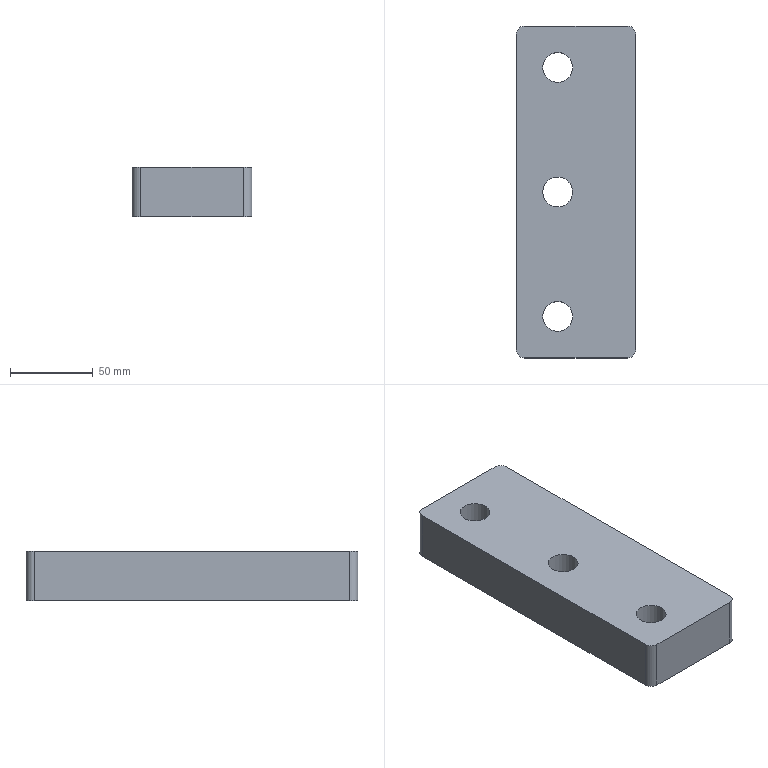Part | NX | features MAIN_BODY 2 | 1 solid | 13 faces | box 72 x 200 x 30 mm | volume 408454 mm3 | cylinder 7 | plane 6 | commonest cylinder face diameters 10 x4 18 x3
STEP:
#1=CARTESIAN_POINT('',(-700.,785.001,85.));
#2=VERTEX_POINT('',#1);
#3=CARTESIAN_POINT('',(-762.,785.001,85.));
#4=VERTEX_POINT('',#3);
#5=CARTESIAN_POINT('',(-695.,785.001,85.));
#6=DIRECTION('',(-1.,0.,0.));
#7=VECTOR('',#6,1000.);
#8=LINE('',#5,#7);
#9=EDGE_CURVE('',#2,#4,#8,.T.);
#10=ORIENTED_EDGE('',*,*,#9,.F.);
#11=CARTESIAN_POINT('',(-700.,785.001,55.));
#12=VERTEX_POINT('',#11);
#13=CARTESIAN_POINT('',(-700.,785.001,55.));
#14=DIRECTION('',(0.,0.,1.));
#15=VECTOR('',#14,1000.);
#16=LINE('',#13,#15);
#17=EDGE_CURVE('',#2,#12,#16,.F.);
#18=ORIENTED_EDGE('',*,*,#17,.T.);
#19=CARTESIAN_POINT('',(-762.,785.001,55.));
#20=VERTEX_POINT('',#19);
#21=CARTESIAN_POINT('',(-695.,785.001,55.));
#22=DIRECTION('',(-1.,0.,0.));
#23=VECTOR('',#22,1000.);
#24=LINE('',#21,#23);
#25=EDGE_CURVE('',#12,#20,#24,.T.);
#26=ORIENTED_EDGE('',*,*,#25,.T.);
#27=CARTESIAN_POINT('',(-762.,785.001,55.));
#28=DIRECTION('',(0.,0.,1.));
#29=VECTOR('',#28,1000.);
#30=LINE('',#27,#29);
#31=EDGE_CURVE('',#20,#4,#30,.T.);
#32=ORIENTED_EDGE('',*,*,#31,.T.);
#33=EDGE_LOOP('',(#10,#18,#26,#32));
#34=FACE_BOUND('',#33,.T.);
#35=CARTESIAN_POINT('',(-695.,785.001,55.));
#36=DIRECTION('',(0.,1.,0.));
#37=DIRECTION('',(1.,0.,0.));
#38=AXIS2_PLACEMENT_3D('',#35,#36,#37);
#39=PLANE('',#38);
#40=ADVANCED_FACE('',(#34),#39,.T.);
#41=CARTESIAN_POINT('',(-767.,780.001,85.));
#42=VERTEX_POINT('',#41);
#43=CARTESIAN_POINT('',(-767.,590.001,85.));
#44=VERTEX_POINT('',#43);
#45=CARTESIAN_POINT('',(-767.,785.001,85.));
#46=DIRECTION('',(0.,-1.,0.));
#47=VECTOR('',#46,1000.);
#48=LINE('',#45,#47);
#49=EDGE_CURVE('',#42,#44,#48,.T.);
#50=ORIENTED_EDGE('',*,*,#49,.F.);
#51=CARTESIAN_POINT('',(-767.,780.001,55.));
#52=VERTEX_POINT('',#51);
#53=CARTESIAN_POINT('',(-767.,780.001,55.));
#54=DIRECTION('',(0.,0.,1.));
#55=VECTOR('',#54,1000.);
#56=LINE('',#53,#55);
#57=EDGE_CURVE('',#42,#52,#56,.F.);
#58=ORIENTED_EDGE('',*,*,#57,.T.);
#59=CARTESIAN_POINT('',(-767.,590.001,55.));
#60=VERTEX_POINT('',#59);
#61=CARTESIAN_POINT('',(-767.,785.001,55.));
#62=DIRECTION('',(0.,-1.,0.));
#63=VECTOR('',#62,1000.);
#64=LINE('',#61,#63);
#65=EDGE_CURVE('',#52,#60,#64,.T.);
#66=ORIENTED_EDGE('',*,*,#65,.T.);
#67=CARTESIAN_POINT('',(-767.,590.001,55.));
#68=DIRECTION('',(0.,0.,1.));
#69=VECTOR('',#68,1000.);
#70=LINE('',#67,#69);
#71=EDGE_CURVE('',#60,#44,#70,.T.);
#72=ORIENTED_EDGE('',*,*,#71,.T.);
#73=EDGE_LOOP('',(#50,#58,#66,#72));
#74=FACE_BOUND('',#73,.T.);
#75=CARTESIAN_POINT('',(-767.,785.001,55.));
#76=DIRECTION('',(-1.,0.,0.));
#77=DIRECTION('',(0.,1.,0.));
#78=AXIS2_PLACEMENT_3D('',#75,#76,#77);
#79=PLANE('',#78);
#80=ADVANCED_FACE('',(#74),#79,.T.);
#81=CARTESIAN_POINT('',(-695.,590.001,55.));
#82=VERTEX_POINT('',#81);
#83=CARTESIAN_POINT('',(-695.,780.001,55.));
#84=VERTEX_POINT('',#83);
#85=CARTESIAN_POINT('',(-695.,685.001,55.));
#86=DIRECTION('',(0.,1.,0.));
#87=VECTOR('',#86,1000.);
#88=LINE('',#85,#87);
#89=EDGE_CURVE('',#82,#84,#88,.T.);
#90=ORIENTED_EDGE('',*,*,#89,.T.);
#91=CARTESIAN_POINT('',(-695.,780.001,85.));
#92=VERTEX_POINT('',#91);
#93=CARTESIAN_POINT('',(-695.,780.001,55.));
#94=DIRECTION('',(0.,0.,1.));
#95=VECTOR('',#94,1000.);
#96=LINE('',#93,#95);
#97=EDGE_CURVE('',#84,#92,#96,.T.);
#98=ORIENTED_EDGE('',*,*,#97,.T.);
#99=CARTESIAN_POINT('',(-695.,590.001,85.));
#100=VERTEX_POINT('',#99);
#101=CARTESIAN_POINT('',(-695.,685.001,85.));
#102=DIRECTION('',(0.,1.,0.));
#103=VECTOR('',#102,1000.);
#104=LINE('',#101,#103);
#105=EDGE_CURVE('',#100,#92,#104,.T.);
#106=ORIENTED_EDGE('',*,*,#105,.F.);
#107=CARTESIAN_POINT('',(-695.,590.001,55.));
#108=DIRECTION('',(0.,0.,1.));
#109=VECTOR('',#108,1000.);
#110=LINE('',#107,#109);
#111=EDGE_CURVE('',#100,#82,#110,.F.);
#112=ORIENTED_EDGE('',*,*,#111,.T.);
#113=EDGE_LOOP('',(#90,#98,#106,#112));
#114=FACE_BOUND('',#113,.T.);
#115=CARTESIAN_POINT('',(-695.,685.001,55.));
#116=DIRECTION('',(1.,0.,0.));
#117=DIRECTION('',(0.,0.,-1.));
#118=AXIS2_PLACEMENT_3D('',#115,#116,#117);
#119=PLANE('',#118);
#120=ADVANCED_FACE('',(#114),#119,.T.);
#121=ORIENTED_EDGE('',*,*,#25,.F.);
#122=CARTESIAN_POINT('',(-700.,780.001,55.));
#123=DIRECTION('',(0.,0.,1.));
#124=DIRECTION('',(0.,-1.,0.));
#125=AXIS2_PLACEMENT_3D('',#122,#123,#124);
#126=CIRCLE('',#125,5.);
#127=EDGE_CURVE('',#12,#84,#126,.F.);
#128=ORIENTED_EDGE('',*,*,#127,.T.);
#129=ORIENTED_EDGE('',*,*,#89,.F.);
#130=CARTESIAN_POINT('',(-700.,585.001,55.));
#131=VERTEX_POINT('',#130);
#132=CARTESIAN_POINT('',(-700.,590.001,55.));
#133=DIRECTION('',(0.,0.,1.));
#134=DIRECTION('',(0.,-1.,0.));
#135=AXIS2_PLACEMENT_3D('',#132,#133,#134);
#136=CIRCLE('',#135,5.);
#137=EDGE_CURVE('',#82,#131,#136,.F.);
#138=ORIENTED_EDGE('',*,*,#137,.T.);
#139=CARTESIAN_POINT('',(-762.,585.001,55.));
#140=VERTEX_POINT('',#139);
#141=CARTESIAN_POINT('',(-695.,585.001,55.));
#142=DIRECTION('',(-1.,0.,0.));
#143=VECTOR('',#142,1000.);
#144=LINE('',#141,#143);
#145=EDGE_CURVE('',#131,#140,#144,.T.);
#146=ORIENTED_EDGE('',*,*,#145,.T.);
#147=CARTESIAN_POINT('',(-762.,590.001,55.));
#148=DIRECTION('',(0.,0.,1.));
#149=DIRECTION('',(0.,-1.,0.));
#150=AXIS2_PLACEMENT_3D('',#147,#148,#149);
#151=CIRCLE('',#150,5.);
#152=EDGE_CURVE('',#140,#60,#151,.F.);
#153=ORIENTED_EDGE('',*,*,#152,.T.);
#154=ORIENTED_EDGE('',*,*,#65,.F.);
#155=CARTESIAN_POINT('',(-762.,780.001,55.));
#156=DIRECTION('',(0.,0.,1.));
#157=DIRECTION('',(0.,-1.,0.));
#158=AXIS2_PLACEMENT_3D('',#155,#156,#157);
#159=CIRCLE('',#158,5.);
#160=EDGE_CURVE('',#52,#20,#159,.F.);
#161=ORIENTED_EDGE('',*,*,#160,.T.);
#162=EDGE_LOOP('',(#121,#128,#129,#138,#146,#153,#154,#161));
#163=FACE_BOUND('',#162,.T.);
#164=CARTESIAN_POINT('',(-742.,751.001,55.));
#165=VERTEX_POINT('',#164);
#166=CARTESIAN_POINT('',(-742.,760.001,55.));
#167=DIRECTION('',(0.,0.,1.));
#168=DIRECTION('',(0.,-1.,0.));
#169=AXIS2_PLACEMENT_3D('',#166,#167,#168);
#170=CIRCLE('',#169,9.);
#171=EDGE_CURVE('',#165,#165,#170,.T.);
#172=ORIENTED_EDGE('',*,*,#171,.T.);
#173=EDGE_LOOP('',(#172));
#174=FACE_BOUND('',#173,.T.);
#175=CARTESIAN_POINT('',(-742.,676.001,55.));
#176=VERTEX_POINT('',#175);
#177=CARTESIAN_POINT('',(-742.,685.001,55.));
#178=DIRECTION('',(0.,0.,1.));
#179=DIRECTION('',(0.,-1.,0.));
#180=AXIS2_PLACEMENT_3D('',#177,#178,#179);
#181=CIRCLE('',#180,9.);
#182=EDGE_CURVE('',#176,#176,#181,.T.);
#183=ORIENTED_EDGE('',*,*,#182,.T.);
#184=EDGE_LOOP('',(#183));
#185=FACE_BOUND('',#184,.T.);
#186=CARTESIAN_POINT('',(-742.,619.001,55.));
#187=VERTEX_POINT('',#186);
#188=CARTESIAN_POINT('',(-742.,610.001,55.));
#189=DIRECTION('',(0.,0.,-1.));
#190=DIRECTION('',(0.,1.,0.));
#191=AXIS2_PLACEMENT_3D('',#188,#189,#190);
#192=CIRCLE('',#191,9.);
#193=EDGE_CURVE('',#187,#187,#192,.T.);
#194=ORIENTED_EDGE('',*,*,#193,.F.);
#195=EDGE_LOOP('',(#194));
#196=FACE_BOUND('',#195,.T.);
#197=CARTESIAN_POINT('',(-767.,785.001,55.));
#198=DIRECTION('',(0.,0.,1.));
#199=DIRECTION('',(0.,-1.,0.));
#200=AXIS2_PLACEMENT_3D('',#197,#198,#199);
#201=PLANE('',#200);
#202=ADVANCED_FACE('',(#163,#174,#185,#196),#201,.F.);
#203=ORIENTED_EDGE('',*,*,#105,.T.);
#204=CARTESIAN_POINT('',(-700.,780.001,85.));
#205=DIRECTION('',(0.,0.,1.));
#206=DIRECTION('',(0.,-1.,0.));
#207=AXIS2_PLACEMENT_3D('',#204,#205,#206);
#208=CIRCLE('',#207,5.);
#209=EDGE_CURVE('',#92,#2,#208,.T.);
#210=ORIENTED_EDGE('',*,*,#209,.T.);
#211=ORIENTED_EDGE('',*,*,#9,.T.);
#212=CARTESIAN_POINT('',(-762.,780.001,85.));
#213=DIRECTION('',(0.,0.,1.));
#214=DIRECTION('',(0.,-1.,0.));
#215=AXIS2_PLACEMENT_3D('',#212,#213,#214);
#216=CIRCLE('',#215,5.);
#217=EDGE_CURVE('',#4,#42,#216,.T.);
#218=ORIENTED_EDGE('',*,*,#217,.T.);
#219=ORIENTED_EDGE('',*,*,#49,.T.);
#220=CARTESIAN_POINT('',(-762.,585.001,85.));
#221=VERTEX_POINT('',#220);
#222=CARTESIAN_POINT('',(-762.,590.001,85.));
#223=DIRECTION('',(0.,0.,1.));
#224=DIRECTION('',(0.,-1.,0.));
#225=AXIS2_PLACEMENT_3D('',#222,#223,#224);
#226=CIRCLE('',#225,5.);
#227=EDGE_CURVE('',#44,#221,#226,.T.);
#228=ORIENTED_EDGE('',*,*,#227,.T.);
#229=CARTESIAN_POINT('',(-700.,585.001,85.));
#230=VERTEX_POINT('',#229);
#231=CARTESIAN_POINT('',(-695.,585.001,85.));
#232=DIRECTION('',(-1.,0.,0.));
#233=VECTOR('',#232,1000.);
#234=LINE('',#231,#233);
#235=EDGE_CURVE('',#230,#221,#234,.T.);
#236=ORIENTED_EDGE('',*,*,#235,.F.);
#237=CARTESIAN_POINT('',(-700.,590.001,85.));
#238=DIRECTION('',(0.,0.,1.));
#239=DIRECTION('',(0.,-1.,0.));
#240=AXIS2_PLACEMENT_3D('',#237,#238,#239);
#241=CIRCLE('',#240,5.);
#242=EDGE_CURVE('',#230,#100,#241,.T.);
#243=ORIENTED_EDGE('',*,*,#242,.T.);
#244=EDGE_LOOP('',(#203,#210,#211,#218,#219,#228,#236,#243));
#245=FACE_BOUND('',#244,.T.);
#246=CARTESIAN_POINT('',(-742.,676.001,85.));
#247=VERTEX_POINT('',#246);
#248=CARTESIAN_POINT('',(-742.,685.001,85.));
#249=DIRECTION('',(0.,0.,1.));
#250=DIRECTION('',(0.,-1.,0.));
#251=AXIS2_PLACEMENT_3D('',#248,#249,#250);
#252=CIRCLE('',#251,9.);
#253=EDGE_CURVE('',#247,#247,#252,.T.);
#254=ORIENTED_EDGE('',*,*,#253,.F.);
#255=EDGE_LOOP('',(#254));
#256=FACE_BOUND('',#255,.T.);
#257=CARTESIAN_POINT('',(-742.,751.001,85.));
#258=VERTEX_POINT('',#257);
#259=CARTESIAN_POINT('',(-742.,760.001,85.));
#260=DIRECTION('',(0.,0.,1.));
#261=DIRECTION('',(0.,-1.,0.));
#262=AXIS2_PLACEMENT_3D('',#259,#260,#261);
#263=CIRCLE('',#262,9.);
#264=EDGE_CURVE('',#258,#258,#263,.T.);
#265=ORIENTED_EDGE('',*,*,#264,.F.);
#266=EDGE_LOOP('',(#265));
#267=FACE_BOUND('',#266,.T.);
#268=CARTESIAN_POINT('',(-742.,619.001,85.));
#269=VERTEX_POINT('',#268);
#270=CARTESIAN_POINT('',(-742.,610.001,85.));
#271=DIRECTION('',(0.,0.,-1.));
#272=DIRECTION('',(0.,1.,0.));
#273=AXIS2_PLACEMENT_3D('',#270,#271,#272);
#274=CIRCLE('',#273,9.);
#275=EDGE_CURVE('',#269,#269,#274,.T.);
#276=ORIENTED_EDGE('',*,*,#275,.T.);
#277=EDGE_LOOP('',(#276));
#278=FACE_BOUND('',#277,.T.);
#279=CARTESIAN_POINT('',(-767.,785.001,85.));
#280=DIRECTION('',(0.,0.,1.));
#281=DIRECTION('',(0.,-1.,0.));
#282=AXIS2_PLACEMENT_3D('',#279,#280,#281);
#283=PLANE('',#282);
#284=ADVANCED_FACE('',(#245,#256,#267,#278),#283,.T.);
#285=ORIENTED_EDGE('',*,*,#264,.T.);
#286=EDGE_LOOP('',(#285));
#287=FACE_BOUND('',#286,.T.);
#288=ORIENTED_EDGE('',*,*,#171,.F.);
#289=EDGE_LOOP('',(#288));
#290=FACE_BOUND('',#289,.T.);
#291=CARTESIAN_POINT('',(-742.,760.001,55.));
#292=DIRECTION('',(0.,0.,1.));
#293=DIRECTION('',(0.,-1.,0.));
#294=AXIS2_PLACEMENT_3D('',#291,#292,#293);
#295=CYLINDRICAL_SURFACE('',#294,9.);
#296=ADVANCED_FACE('',(#287,#290),#295,.F.);
#297=ORIENTED_EDGE('',*,*,#253,.T.);
#298=EDGE_LOOP('',(#297));
#299=FACE_BOUND('',#298,.T.);
#300=ORIENTED_EDGE('',*,*,#182,.F.);
#301=EDGE_LOOP('',(#300));
#302=FACE_BOUND('',#301,.T.);
#303=CARTESIAN_POINT('',(-742.,685.001,55.));
#304=DIRECTION('',(0.,0.,1.));
#305=DIRECTION('',(0.,-1.,0.));
#306=AXIS2_PLACEMENT_3D('',#303,#304,#305);
#307=CYLINDRICAL_SURFACE('',#306,9.);
#308=ADVANCED_FACE('',(#299,#302),#307,.F.);
#309=ORIENTED_EDGE('',*,*,#145,.F.);
#310=CARTESIAN_POINT('',(-700.,585.001,55.));
#311=DIRECTION('',(0.,0.,1.));
#312=VECTOR('',#311,1000.);
#313=LINE('',#310,#312);
#314=EDGE_CURVE('',#131,#230,#313,.T.);
#315=ORIENTED_EDGE('',*,*,#314,.T.);
#316=ORIENTED_EDGE('',*,*,#235,.T.);
#317=CARTESIAN_POINT('',(-762.,585.001,55.));
#318=DIRECTION('',(0.,0.,1.));
#319=VECTOR('',#318,1000.);
#320=LINE('',#317,#319);
#321=EDGE_CURVE('',#221,#140,#320,.F.);
#322=ORIENTED_EDGE('',*,*,#321,.T.);
#323=EDGE_LOOP('',(#309,#315,#316,#322));
#324=FACE_BOUND('',#323,.T.);
#325=CARTESIAN_POINT('',(-695.,585.001,55.));
#326=DIRECTION('',(0.,-1.,0.));
#327=DIRECTION('',(1.,0.,0.));
#328=AXIS2_PLACEMENT_3D('',#325,#326,#327);
#329=PLANE('',#328);
#330=ADVANCED_FACE('',(#324),#329,.T.);
#331=ORIENTED_EDGE('',*,*,#275,.F.);
#332=EDGE_LOOP('',(#331));
#333=FACE_BOUND('',#332,.T.);
#334=ORIENTED_EDGE('',*,*,#193,.T.);
#335=EDGE_LOOP('',(#334));
#336=FACE_BOUND('',#335,.T.);
#337=CARTESIAN_POINT('',(-742.,610.001,55.));
#338=DIRECTION('',(0.,0.,1.));
#339=DIRECTION('',(0.,1.,0.));
#340=AXIS2_PLACEMENT_3D('',#337,#338,#339);
#341=CYLINDRICAL_SURFACE('',#340,9.);
#342=ADVANCED_FACE('',(#333,#336),#341,.F.);
#343=ORIENTED_EDGE('',*,*,#127,.F.);
#344=ORIENTED_EDGE('',*,*,#17,.F.);
#345=ORIENTED_EDGE('',*,*,#209,.F.);
#346=ORIENTED_EDGE('',*,*,#97,.F.);
#347=EDGE_LOOP('',(#343,#344,#345,#346));
#348=FACE_BOUND('',#347,.T.);
#349=CARTESIAN_POINT('',(-700.,780.001,55.));
#350=DIRECTION('',(0.,0.,1.));
#351=DIRECTION('',(0.,-1.,0.));
#352=AXIS2_PLACEMENT_3D('',#349,#350,#351);
#353=CYLINDRICAL_SURFACE('',#352,5.);
#354=ADVANCED_FACE('',(#348),#353,.T.);
#355=ORIENTED_EDGE('',*,*,#160,.F.);
#356=ORIENTED_EDGE('',*,*,#57,.F.);
#357=ORIENTED_EDGE('',*,*,#217,.F.);
#358=ORIENTED_EDGE('',*,*,#31,.F.);
#359=EDGE_LOOP('',(#355,#356,#357,#358));
#360=FACE_BOUND('',#359,.T.);
#361=CARTESIAN_POINT('',(-762.,780.001,55.));
#362=DIRECTION('',(0.,0.,1.));
#363=DIRECTION('',(0.,-1.,0.));
#364=AXIS2_PLACEMENT_3D('',#361,#362,#363);
#365=CYLINDRICAL_SURFACE('',#364,5.);
#366=ADVANCED_FACE('',(#360),#365,.T.);
#367=ORIENTED_EDGE('',*,*,#137,.F.);
#368=ORIENTED_EDGE('',*,*,#111,.F.);
#369=ORIENTED_EDGE('',*,*,#242,.F.);
#370=ORIENTED_EDGE('',*,*,#314,.F.);
#371=EDGE_LOOP('',(#367,#368,#369,#370));
#372=FACE_BOUND('',#371,.T.);
#373=CARTESIAN_POINT('',(-700.,590.001,55.));
#374=DIRECTION('',(0.,0.,1.));
#375=DIRECTION('',(0.,-1.,0.));
#376=AXIS2_PLACEMENT_3D('',#373,#374,#375);
#377=CYLINDRICAL_SURFACE('',#376,5.);
#378=ADVANCED_FACE('',(#372),#377,.T.);
#379=ORIENTED_EDGE('',*,*,#152,.F.);
#380=ORIENTED_EDGE('',*,*,#321,.F.);
#381=ORIENTED_EDGE('',*,*,#227,.F.);
#382=ORIENTED_EDGE('',*,*,#71,.F.);
#383=EDGE_LOOP('',(#379,#380,#381,#382));
#384=FACE_BOUND('',#383,.T.);
#385=CARTESIAN_POINT('',(-762.,590.001,55.));
#386=DIRECTION('',(0.,0.,1.));
#387=DIRECTION('',(0.,-1.,0.));
#388=AXIS2_PLACEMENT_3D('',#385,#386,#387);
#389=CYLINDRICAL_SURFACE('',#388,5.);
#390=ADVANCED_FACE('',(#384),#389,.T.);
#391=CLOSED_SHELL('',(#40,#80,#120,#202,#284,#296,#308,#330,#342,#354,#366,#378,#390));
#392=MANIFOLD_SOLID_BREP('',#391);
#393=(LENGTH_UNIT()NAMED_UNIT(*)SI_UNIT(.MILLI.,.METRE.));
#394=UNCERTAINTY_MEASURE_WITH_UNIT(LENGTH_MEASURE(0.00001),#393,'','');
#395=(NAMED_UNIT(*)PLANE_ANGLE_UNIT()SI_UNIT($,.RADIAN.));
#396=(NAMED_UNIT(*)SI_UNIT($,.STERADIAN.)SOLID_ANGLE_UNIT());
#397=(GEOMETRIC_REPRESENTATION_CONTEXT(3)GLOBAL_UNCERTAINTY_ASSIGNED_CONTEXT((#394))GLOBAL_UNIT_ASSIGNED_CONTEXT((#393,#395,#396))REPRESENTATION_CONTEXT('',''));
#398=ADVANCED_BREP_SHAPE_REPRESENTATION('',(#392),#397);